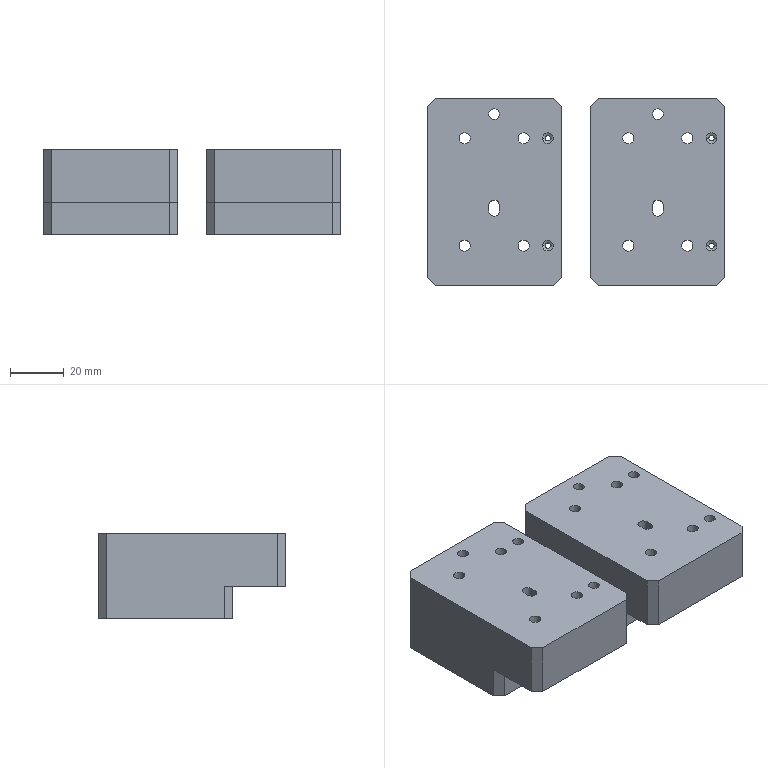NC program | NX | posted with a generic post | part box 111 x 70 x 32 mm
Lines 4642 to 5357 of 5357:
(ZLEVEL_PROFILE_1 , TOOL : D10JING)
N9276 T14 M6
N9278 G54
N9280 G17 G0 G90 X117.809 Y68.622 S9500 M3
N9282 G43 Z30. H14
N9284 Z-14.5
N9286 G94 G1 Z-16. F1000.
N9288 X116.5 Y67.866
N9290 G3 X116. Y67. R1.
N9292 G1 Y3. F1500.
N9294 G2 X114.536 Y-0.536 R5.
N9296 G1 X111.536 Y-3.536
N9298 G2 X108. Y-5. R5.
N9300 G1 X64.
N9302 G2 X60.464 Y-3.536 R5.
N9304 G1 X57.464 Y-0.536
N9306 G2 X56. Y3. R5.
N9308 G1 Y67.
N9310 G2 X57.464 Y70.536 R5.
N9312 G1 X60.464 Y73.536
N9314 G2 X64. Y75. R5.
N9316 G1 X108.
N9318 G2 X111.536 Y73.536 R5.
N9320 G1 X114.536 Y70.536
N9322 G2 X116. Y67. R5.
N9324 G3 X116.5 Y66.134 R1.
N9326 G1 X118. Y65.268
N9328 Z-14.5
N9330 G0 Z53.
N9332 X-6.809 Y1.378
N9334 Z-14.5
N9336 G1 Z-16. F1000.
N9338 X-5.5 Y2.134
N9340 G3 X-5. Y3. R1.
N9342 G1 Y67. F1500.
N9344 G2 X-3.536 Y70.536 R5.
N9346 G1 X-0.536 Y73.536
N9348 G2 X3. Y75. R5.
N9350 G1 X47.
N9352 G2 X50.536 Y73.536 R5.
N9354 G1 X53.536 Y70.536
N9356 G2 X55. Y67. R5.
N9358 G1 Y3.
N9360 G2 X53.536 Y-0.536 R5.
N9362 G1 X50.536 Y-3.536
N9364 G2 X47. Y-5. R5.
N9366 G1 X3.
N9368 G2 X-0.536 Y-3.536 R5.
N9370 G1 X-3.536 Y-0.536
N9372 G2 X-5. Y3. R5.
N9374 G1 Y67. Z-19.873
N9376 X-4.992 Y67.28 Z-19.89
N9378 X-4.969 Y67.56 Z-19.907
N9380 X-4.929 Y67.838 Z-19.924
N9382 X-4.875 Y68.113 Z-19.941
N9384 X-4.805 Y68.384 Z-19.958
N9386 X-4.719 Y68.651 Z-19.975
N9388 X-4.619 Y68.913 Z-19.992
N9390 X-4.505 Y69.169 Z-20.009
N9392 X-4.376 Y69.419 Z-20.026
N9394 X-4.234 Y69.66 Z-20.043
N9396 X-4.078 Y69.893 Z-20.06
N9398 X-3.909 Y70.117 Z-20.077
N9400 X-3.728 Y70.332 Z-20.094
N9402 X-3.536 Y70.536 Z-20.111
N9404 X-0.536 Y73.536 Z-20.368
N9406 X-0.332 Y73.728 Z-20.385
N9408 X-0.117 Y73.909 Z-20.402
N9410 X0.107 Y74.078 Z-20.419
N9412 X0.34 Y74.234 Z-20.436
N9414 X0.581 Y74.376 Z-20.453
N9416 X0.831 Y74.505 Z-20.469
N9418 X1.087 Y74.619 Z-20.486
N9420 X1.349 Y74.719 Z-20.503
N9422 X1.616 Y74.805 Z-20.52
N9424 X1.887 Y74.875 Z-20.537
N9426 X2.162 Y74.929 Z-20.554
N9428 X2.44 Y74.969 Z-20.571
N9430 X2.72 Y74.992 Z-20.588
N9432 X3. Y75. Z-20.605
N9434 X47. Z-23.268
N9436 X47.28 Y74.992 Z-23.285
N9438 X47.56 Y74.969 Z-23.302
N9440 X47.838 Y74.929 Z-23.319
N9442 X48.113 Y74.875 Z-23.336
N9444 X48.384 Y74.805 Z-23.353
N9446 X48.651 Y74.719 Z-23.37
N9448 X48.913 Y74.619 Z-23.387
N9450 X49.169 Y74.505 Z-23.404
N9452 X49.419 Y74.376 Z-23.421
N9454 X49.66 Y74.234 Z-23.438
N9456 X49.893 Y74.078 Z-23.455
N9458 X50.117 Y73.909 Z-23.472
N9460 X50.332 Y73.728 Z-23.489
N9462 X50.536 Y73.536 Z-23.506
N9464 X53.536 Y70.536 Z-23.762
N9466 X53.728 Y70.332 Z-23.779
N9468 X53.909 Y70.117 Z-23.796
N9470 X54.078 Y69.893 Z-23.813
N9472 X54.234 Y69.66 Z-23.83
N9474 X54.376 Y69.419 Z-23.847
N9476 X54.505 Y69.169 Z-23.864
N9478 X54.619 Y68.913 Z-23.881
N9480 X54.719 Y68.651 Z-23.898
N9482 X54.805 Y68.384 Z-23.915
N9484 X54.875 Y68.113 Z-23.932
N9486 X54.929 Y67.838 Z-23.949
N9488 X54.969 Y67.56 Z-23.966
N9490 X54.992 Y67.28 Z-23.983
N9492 X55. Y67. Z-24.
N9494 Y3. Z-27.873
N9496 X54.992 Y2.72 Z-27.89
N9498 X54.969 Y2.44 Z-27.907
N9500 X54.929 Y2.162 Z-27.924
N9502 X54.875 Y1.887 Z-27.941
N9504 X54.805 Y1.616 Z-27.958
N9506 X54.719 Y1.349 Z-27.975
N9508 X54.619 Y1.087 Z-27.992
N9510 X54.505 Y0.831 Z-28.009
N9512 X54.376 Y0.581 Z-28.026
N9514 X54.234 Y0.34 Z-28.043
N9516 X54.078 Y0.107 Z-28.06
N9518 X53.909 Y-0.117 Z-28.077
N9520 X53.728 Y-0.332 Z-28.094
N9522 X53.536 Y-0.536 Z-28.111
N9524 X50.536 Y-3.536 Z-28.368
N9526 X50.332 Y-3.728 Z-28.385
N9528 X50.117 Y-3.909 Z-28.402
N9530 X49.893 Y-4.078 Z-28.419
N9532 X49.66 Y-4.234 Z-28.436
N9534 X49.419 Y-4.376 Z-28.453
N9536 X49.169 Y-4.505 Z-28.469
N9538 X48.913 Y-4.619 Z-28.486
N9540 X48.651 Y-4.719 Z-28.503
N9542 X48.384 Y-4.805 Z-28.52
N9544 X48.113 Y-4.875 Z-28.537
N9546 X47.838 Y-4.929 Z-28.554
N9548 X47.56 Y-4.969 Z-28.571
N9550 X47.28 Y-4.992 Z-28.588
N9552 X47. Y-5. Z-28.605
N9554 X3. Z-31.268
N9556 X2.72 Y-4.992 Z-31.285
N9558 X2.44 Y-4.969 Z-31.302
N9560 X2.162 Y-4.929 Z-31.319
N9562 X1.887 Y-4.875 Z-31.336
N9564 X1.616 Y-4.805 Z-31.353
N9566 X1.349 Y-4.719 Z-31.37
N9568 X1.087 Y-4.619 Z-31.387
N9570 X0.831 Y-4.505 Z-31.404
N9572 X0.581 Y-4.376 Z-31.421
N9574 X0.34 Y-4.234 Z-31.438
N9576 X0.107 Y-4.078 Z-31.455
N9578 X-0.117 Y-3.909 Z-31.472
N9580 X-0.332 Y-3.728 Z-31.489
N9582 X-0.536 Y-3.536 Z-31.506
N9584 X-3.536 Y-0.536 Z-31.762
N9586 X-3.728 Y-0.332 Z-31.779
N9588 X-3.909 Y-0.117 Z-31.796
N9590 X-4.078 Y0.107 Z-31.813
N9592 X-4.234 Y0.34 Z-31.83
N9594 X-4.376 Y0.581 Z-31.847
N9596 X-4.505 Y0.831 Z-31.864
N9598 X-4.619 Y1.087 Z-31.881
N9600 X-4.719 Y1.349 Z-31.898
N9602 X-4.805 Y1.616 Z-31.915
N9604 X-4.875 Y1.887 Z-31.932
N9606 X-4.929 Y2.162 Z-31.949
N9608 X-4.969 Y2.44 Z-31.966
N9610 X-4.992 Y2.72 Z-31.983
N9612 X-5. Y3. Z-32.
N9614 Y67.
N9616 G2 X-3.536 Y70.536 R5.
N9618 G1 X-0.536 Y73.536
N9620 G2 X3. Y75. R5.
N9622 G1 X47.
N9624 G2 X50.536 Y73.536 R5.
N9626 G1 X53.536 Y70.536
N9628 G2 X55. Y67. R5.
N9630 G1 Y3.
N9632 G2 X53.536 Y-0.536 R5.
N9634 G1 X50.536 Y-3.536
N9636 G2 X47. Y-5. R5.
N9638 G1 X3.
N9640 G2 X-0.536 Y-3.536 R5.
N9642 G1 X-3.536 Y-0.536
N9644 G2 X-5. Y3. R5.
N9646 G3 X-5.5 Y3.866 R1.
N9648 G1 X-7. Y4.732
N9650 Z-30.5
N9652 G0 Z53.
N9654 X117.809 Y68.622
N9656 Z-30.5
N9658 G1 Z-32. F1000.
N9660 X116.5 Y67.866
N9662 G3 X116. Y67. R1.
N9664 G1 Y3. F1500.
N9666 G2 X114.536 Y-0.536 R5.
N9668 G1 X111.536 Y-3.536
N9670 G2 X108. Y-5. R5.
N9672 G1 X64.
N9674 G2 X60.464 Y-3.536 R5.
N9676 G1 X57.464 Y-0.536
N9678 G2 X56. Y3. R5.
N9680 G1 Y67.
N9682 G2 X57.464 Y70.536 R5.
N9684 G1 X60.464 Y73.536
N9686 G2 X64. Y75. R5.
N9688 G1 X108.
N9690 G2 X111.536 Y73.536 R5.
N9692 G1 X114.536 Y70.536
N9694 G2 X116. Y67. R5.
N9696 G3 X116.5 Y66.134 R1.
N9698 G1 X118. Y65.268
N9700 Z-30.5
N9702 G0 Z30.
N9704 M5
(DRILLING , TOOL : D6A45)
N9706 T01 M6
N9708 G54
N9710 G17 G0 G90 X106. Y55. S9500 M3
N9712 G43 Z30. H1
N9714 G94 G81 G98 Z-1.8 F250. R3.
N9716 X97.
N9718 X86. Y64.
N9720 X75. Y55.
N9722 X45.
N9724 X36.
N9726 X25. Y64.
N9728 X14. Y55.
N9730 X25. Y28.
N9732 X14. Y15.
N9734 X36.
N9736 X45.
N9738 X75.
N9740 X86. Y28.
N9742 X97. Y15.
N9744 X106.
N9746 G80
N9748 G0 X106. Y15. Z30.
N9750 M5
(DRILLING_COPY_COPY , TOOL : 4.2ZT)
N9752 T04 M6
N9754 G54
N9756 G17 G0 G90 X14. Y15. S2000 M3
N9758 G43 Z30. H4
N9760 G94 G83 G98 Z-22.762 F150. Q2. R3.
N9762 X36.
N9764 X75.
N9766 X97.
N9768 Y55. Z-34.762
N9770 X75.
N9772 X36.
N9774 X14.
N9776 G80
N9778 G0 X14. Y55. Z30.
N9780 M5
(DRILLING_COPY_COPY_1 , TOOL : 3.4ZT)
N9782 T18 M6
N9784 G54
N9786 G17 G0 G90 X25. Y64. S2000 M3
N9788 G43 Z30. H18
N9790 G94 G83 G98 Z-34.521 F150. Q2. R3.
N9792 Y28.
N9794 X45. Y15. Z-8.202
N9796 Y55.
N9798 X86. Y28. Z-34.521
N9800 Y64.
N9802 X106. Y55. Z-8.202
N9804 Y15.
N9806 G80
N9808 G0 X106. Y15. Z30.
N9810 M5
(DRILLING_COPY_COPY_1_COPY , TOOL : 2.0ZT)
N9812 T17 M6
N9814 G54
N9816 G17 G0 G90 X45. Y15. S2000 M3
N9818 G43 Z30. H17
N9820 G94 G83 G98 Z-22.101 F80. Q2. R3.
N9822 Y55. Z-34.101
N9824 X106. Y15. Z-22.101
N9826 Y55. Z-34.101
N9828 G80
N9830 G0 X106. Y55. Z30.
N9832 M5
(HOLE_MILLING , TOOL : D3)
N9834 T03 M6
N9836 G54
N9838 G17 G0 G90 X45. Y55. S9500 M3
N9840 G43 Z30. H3
N9842 Z0.5
N9844 G94 G3 X45.2 Y54.8 R0.2 F1250.
N9846 X45.4 Y55. R0.2
N9848 X45.4 Y55. Z0.3 I-0.4 J0.
N9850 X45.4 Y55. Z0.1 I-0.4 J0.
N9852 X45.4 Y55. Z-0.1 I-0.4 J0.
N9854 X45.4 Y55. Z-0.3 I-0.4 J0.
N9856 X45.4 Y55. Z-0.5 I-0.4 J0.
N9858 X45.4 Y55. Z-0.7 I-0.4 J0.
N9860 X45.4 Y55. Z-0.9 I-0.4 J0.
N9862 X45.4 Y55. Z-1.1 I-0.4 J0.
N9864 X45.4 Y55. Z-1.3 I-0.4 J0.
N9866 X45.4 Y55. Z-1.5 I-0.4 J0.
N9868 X45.4 Y55. Z-1.7 I-0.4 J0.
N9870 X45.4 Y55. Z-1.9 I-0.4 J0.
N9872 X45.4 Y55. Z-2.1 I-0.4 J0.
N9874 X45.4 Y55. Z-2.3 I-0.4 J0.
N9876 X45.4 Y55. Z-2.5 I-0.4 J0.
N9878 X45.4 Y55. Z-2.7 I-0.4 J0.
N9880 X45.4 Y55. Z-2.9 I-0.4 J0.
N9882 X45.4 Y55. Z-3.1 I-0.4 J0.
N9884 X45.4 Y55. Z-3.3 I-0.4 J0.
N9886 X45.4 Y55. Z-3.5 I-0.4 J0.
N9888 X45.4 Y55. Z-3.7 I-0.4 J0.
N9890 X45.4 Y55. Z-3.9 I-0.4 J0.
N9892 X45.4 Y55. Z-4.1 I-0.4 J0.
N9894 X45.4 Y55. Z-4.3 I-0.4 J0.
N9896 X45.4 Y55. Z-4.5 I-0.4 J0.
N9898 X45.4 Y55. Z-4.7 I-0.4 J0.
N9900 X45.4 Y55. Z-4.9 I-0.4 J0.
N9902 X45.4 Y55. Z-5.1 I-0.4 J0.
N9904 X45.4 Y55. Z-5.3 I-0.4 J0.
N9906 X45.4 Y55. Z-5.5 I-0.4 J0.
N9908 X45.4 Y55. Z-5.7 I-0.4 J0.
N9910 X45.4 Y55. Z-5.9 I-0.4 J0.
N9912 X45.4 Y55. Z-6.1 I-0.4 J0.
N9914 X45.4 Y55. Z-6.3 I-0.4 J0.
N9916 X45.4 Y55. Z-6.5 I-0.4 J0.
N9918 X45.4 Y55. Z-6.7 I-0.4 J0.
N9920 X45.4 Y55. Z-6.9 I-0.4 J0.
N9922 X44.6 Y55. Z-7. I-0.4 J0.
N9924 X45. Y54.6 R0.4
N9926 X44.6 Y55. R-0.4
N9928 X44.8 Y54.8 R0.2
N9930 X45. Y55. R0.2
N9932 G0 Z30.
N9934 Y15.
N9936 Z0.5
N9938 G3 X45.2 Y14.8 R0.2
N9940 X45.4 Y15. R0.2
N9942 X45.4 Y15. Z0.3 I-0.4 J0.
N9944 X45.4 Y15. Z0.1 I-0.4 J0.
N9946 X45.4 Y15. Z-0.1 I-0.4 J0.
N9948 X45.4 Y15. Z-0.3 I-0.4 J0.
N9950 X45.4 Y15. Z-0.5 I-0.4 J0.
N9952 X45.4 Y15. Z-0.7 I-0.4 J0.
N9954 X45.4 Y15. Z-0.9 I-0.4 J0.
N9956 X45.4 Y15. Z-1.1 I-0.4 J0.
N9958 X45.4 Y15. Z-1.3 I-0.4 J0.
N9960 X45.4 Y15. Z-1.5 I-0.4 J0.
N9962 X45.4 Y15. Z-1.7 I-0.4 J0.
N9964 X45.4 Y15. Z-1.9 I-0.4 J0.
N9966 X45.4 Y15. Z-2.1 I-0.4 J0.
N9968 X45.4 Y15. Z-2.3 I-0.4 J0.
N9970 X45.4 Y15. Z-2.5 I-0.4 J0.
N9972 X45.4 Y15. Z-2.7 I-0.4 J0.
N9974 X45.4 Y15. Z-2.9 I-0.4 J0.
N9976 X45.4 Y15. Z-3.1 I-0.4 J0.
N9978 X45.4 Y15. Z-3.3 I-0.4 J0.
N9980 X45.4 Y15. Z-3.5 I-0.4 J0.
N9982 X45.4 Y15. Z-3.7 I-0.4 J0.
N9984 X45.4 Y15. Z-3.9 I-0.4 J0.
N9986 X45.4 Y15. Z-4.1 I-0.4 J0.
N9988 X45.4 Y15. Z-4.3 I-0.4 J0.
N9990 X45.4 Y15. Z-4.5 I-0.4 J0.
N9992 X45.4 Y15. Z-4.7 I-0.4 J0.
N9994 X45.4 Y15. Z-4.9 I-0.4 J0.
N9996 X45.4 Y15. Z-5.1 I-0.4 J0.
N9998 X45.4 Y15. Z-5.3 I-0.4 J0.
N10000 X45.4 Y15. Z-5.5 I-0.4 J0.
N10002 X45.4 Y15. Z-5.7 I-0.4 J0.
N10004 X45.4 Y15. Z-5.9 I-0.4 J0.
N10006 X45.4 Y15. Z-6.1 I-0.4 J0.
N10008 X45.4 Y15. Z-6.3 I-0.4 J0.
N10010 X45.4 Y15. Z-6.5 I-0.4 J0.
N10012 X45.4 Y15. Z-6.7 I-0.4 J0.
N10014 X45.4 Y15. Z-6.9 I-0.4 J0.
N10016 X44.6 Y15. Z-7. I-0.4 J0.
N10018 X45. Y14.6 R0.4
N10020 X44.6 Y15. R-0.4
N10022 X44.8 Y14.8 R0.2
N10024 X45. Y15. R0.2
N10026 G0 Z30.
N10028 X106.
N10030 Z0.5
N10032 G3 X106.2 Y14.8 R0.2
N10034 X106.4 Y15. R0.2
N10036 X106.4 Y15. Z0.3 I-0.4 J0.
N10038 X106.4 Y15. Z0.1 I-0.4 J0.
N10040 X106.4 Y15. Z-0.1 I-0.4 J0.
N10042 X106.4 Y15. Z-0.3 I-0.4 J0.
N10044 X106.4 Y15. Z-0.5 I-0.4 J0.
N10046 X106.4 Y15. Z-0.7 I-0.4 J0.
N10048 X106.4 Y15. Z-0.9 I-0.4 J0.
N10050 X106.4 Y15. Z-1.1 I-0.4 J0.
N10052 X106.4 Y15. Z-1.3 I-0.4 J0.
N10054 X106.4 Y15. Z-1.5 I-0.4 J0.
N10056 X106.4 Y15. Z-1.7 I-0.4 J0.
N10058 X106.4 Y15. Z-1.9 I-0.4 J0.
N10060 X106.4 Y15. Z-2.1 I-0.4 J0.
N10062 X106.4 Y15. Z-2.3 I-0.4 J0.
N10064 X106.4 Y15. Z-2.5 I-0.4 J0.
N10066 X106.4 Y15. Z-2.7 I-0.4 J0.
N10068 X106.4 Y15. Z-2.9 I-0.4 J0.
N10070 X106.4 Y15. Z-3.1 I-0.4 J0.
N10072 X106.4 Y15. Z-3.3 I-0.4 J0.
N10074 X106.4 Y15. Z-3.5 I-0.4 J0.
N10076 X106.4 Y15. Z-3.7 I-0.4 J0.
N10078 X106.4 Y15. Z-3.9 I-0.4 J0.
N10080 X106.4 Y15. Z-4.1 I-0.4 J0.
N10082 X106.4 Y15. Z-4.3 I-0.4 J0.
N10084 X106.4 Y15. Z-4.5 I-0.4 J0.
N10086 X106.4 Y15. Z-4.7 I-0.4 J0.
N10088 X106.4 Y15. Z-4.9 I-0.4 J0.
N10090 X106.4 Y15. Z-5.1 I-0.4 J0.
N10092 X106.4 Y15. Z-5.3 I-0.4 J0.
N10094 X106.4 Y15. Z-5.5 I-0.4 J0.
N10096 X106.4 Y15. Z-5.7 I-0.4 J0.
N10098 X106.4 Y15. Z-5.9 I-0.4 J0.
N10100 X106.4 Y15. Z-6.1 I-0.4 J0.
N10102 X106.4 Y15. Z-6.3 I-0.4 J0.
N10104 X106.4 Y15. Z-6.5 I-0.4 J0.
N10106 X106.4 Y15. Z-6.7 I-0.4 J0.
N10108 X106.4 Y15. Z-6.9 I-0.4 J0.
N10110 X105.6 Y15. Z-7. I-0.4 J0.
N10112 X106. Y14.6 R0.4
N10114 X105.6 Y15. R-0.4
N10116 X105.8 Y14.8 R0.2
N10118 X106. Y15. R0.2
N10120 G0 Z30.
N10122 Y55.
N10124 Z0.5
N10126 G3 X106.2 Y54.8 R0.2
N10128 X106.4 Y55. R0.2
N10130 X106.4 Y55. Z0.3 I-0.4 J0.
N10132 X106.4 Y55. Z0.1 I-0.4 J0.
N10134 X106.4 Y55. Z-0.1 I-0.4 J0.
N10136 X106.4 Y55. Z-0.3 I-0.4 J0.
N10138 X106.4 Y55. Z-0.5 I-0.4 J0.
N10140 X106.4 Y55. Z-0.7 I-0.4 J0.
N10142 X106.4 Y55. Z-0.9 I-0.4 J0.
N10144 X106.4 Y55. Z-1.1 I-0.4 J0.
N10146 X106.4 Y55. Z-1.3 I-0.4 J0.
N10148 X106.4 Y55. Z-1.5 I-0.4 J0.
N10150 X106.4 Y55. Z-1.7 I-0.4 J0.
N10152 X106.4 Y55. Z-1.9 I-0.4 J0.
N10154 X106.4 Y55. Z-2.1 I-0.4 J0.
N10156 X106.4 Y55. Z-2.3 I-0.4 J0.
N10158 X106.4 Y55. Z-2.5 I-0.4 J0.
N10160 X106.4 Y55. Z-2.7 I-0.4 J0.
N10162 X106.4 Y55. Z-2.9 I-0.4 J0.
N10164 X106.4 Y55. Z-3.1 I-0.4 J0.
N10166 X106.4 Y55. Z-3.3 I-0.4 J0.
N10168 X106.4 Y55. Z-3.5 I-0.4 J0.
N10170 X106.4 Y55. Z-3.7 I-0.4 J0.
N10172 X106.4 Y55. Z-3.9 I-0.4 J0.
N10174 X106.4 Y55. Z-4.1 I-0.4 J0.
N10176 X106.4 Y55. Z-4.3 I-0.4 J0.
N10178 X106.4 Y55. Z-4.5 I-0.4 J0.
N10180 X106.4 Y55. Z-4.7 I-0.4 J0.
N10182 X106.4 Y55. Z-4.9 I-0.4 J0.
N10184 X106.4 Y55. Z-5.1 I-0.4 J0.
N10186 X106.4 Y55. Z-5.3 I-0.4 J0.
N10188 X106.4 Y55. Z-5.5 I-0.4 J0.
N10190 X106.4 Y55. Z-5.7 I-0.4 J0.
N10192 X106.4 Y55. Z-5.9 I-0.4 J0.
N10194 X106.4 Y55. Z-6.1 I-0.4 J0.
N10196 X106.4 Y55. Z-6.3 I-0.4 J0.
N10198 X106.4 Y55. Z-6.5 I-0.4 J0.
N10200 X106.4 Y55. Z-6.7 I-0.4 J0.
N10202 X106.4 Y55. Z-6.9 I-0.4 J0.
N10204 X105.6 Y55. Z-7. I-0.4 J0.
N10206 X106. Y54.6 R0.4
N10208 X105.6 Y55. R-0.4
N10210 X105.8 Y54.8 R0.2
N10212 X106. Y55. R0.2
N10214 G0 Z30.
N10216 M5
(PLANAR_MILL_COPY , TOOL : D6A45)
N10218 T01 M6
N10220 G54
N10222 G17 G0 G90 X44.134 Y14.4 S9500 M3
N10224 G43 Z30. H1
N10226 Z0.5
N10228 G94 G1 Z-1. F1250.
N10230 G3 X45. Y13.9 R1.
N10232 X46.1 Y15. R1.1
N10234 X45. Y13.9 R-1.1
N10236 X45.866 Y14.4 R1.
N10238 G1 Z0.5
N10240 G0 Z30.
N10242 X35.134 Y14.3
N10244 Z0.5
N10246 G1 Z-1.
N10248 G3 X36. Y13.8 R1.
N10250 X37.2 Y15. R1.2
N10252 X36. Y13.8 R-1.2
N10254 X36.866 Y14.3 R1.
N10256 G1 Z0.5
N10258 G0 Z30.
N10260 X13.3 Y15.866
N10262 Z0.5
N10264 G1 Z-1.
N10266 G3 X12.8 Y15. R1.
N10268 X14. Y13.8 R1.2
N10270 X12.8 Y15. R-1.2
N10272 X13.3 Y14.134 R1.
N10274 G1 Z0.5
N10276 G0 Z30.
N10278 X-1.4 Y34.134
N10280 Z0.5
N10282 G1 Z-1.
N10284 G3 X-0.9 Y35. R1.
N10286 G1 Y67.
N10288 G2 X-0.636 Y67.636 R0.9
N10290 G1 X2.364 Y70.636
N10292 G2 X3. Y70.9 R0.9
N10294 G1 X47.
N10296 G2 X47.636 Y70.636 R0.9
N10298 G1 X50.636 Y67.636
N10300 G2 X50.9 Y67. R0.9
N10302 G1 Y3.
N10304 G2 X50.636 Y2.364 R0.9
N10306 G1 X47.636 Y-0.636
N10308 G2 X47. Y-0.9 R0.9
N10310 G1 X3.
N10312 G2 X2.364 Y-0.636 R0.9
N10314 G1 X-0.636 Y2.364
N10316 G2 X-0.9 Y3. R0.9
N10318 G1 Y35.
N10320 G3 X-1.4 Y35.866 R1.
N10322 G1 Z0.5
N10324 G0 Z30.
N10326 X13.3 Y55.866
N10328 Z0.5
N10330 G1 Z-1.
N10332 G3 X12.8 Y55. R1.
N10334 X14. Y53.8 R1.2
N10336 X12.8 Y55. R-1.2
N10338 X13.3 Y54.134 R1.
N10340 G1 Z0.5
N10342 G0 Z30.
N10344 X36.866 Y55.7
N10346 Z0.5
N10348 G1 Z-1.
N10350 G3 X36. Y56.2 R1.
N10352 X34.8 Y55. R1.2
N10354 X36. Y56.2 R-1.2
N10356 X35.134 Y55.7 R1.
N10358 G1 Z0.5
N10360 G0 Z30.
N10362 X45.866 Y55.6
N10364 Z0.5
N10366 G1 Z-1.
N10368 G3 X45. Y56.1 R1.
N10370 X43.9 Y55. R1.1
N10372 X45. Y56.1 R-1.1
N10374 X44.134 Y55.6 R1.
N10376 G1 Z0.5
N10378 G0 Z30.
N10380 X75.866 Y55.7
N10382 Z0.5
N10384 G1 Z-1.
N10386 G3 X75. Y56.2 R1.
N10388 X73.8 Y55. R1.2
N10390 X75. Y56.2 R-1.2
N10392 X74.134 Y55.7 R1.
N10394 G1 Z0.5
N10396 G0 Z30.
N10398 X97.7 Y54.134
N10400 Z0.5
N10402 G1 Z-1.
N10404 G3 X98.2 Y55. R1.
N10406 X97. Y56.2 R1.2
N10408 X98.2 Y55. R-1.2
N10410 X97.7 Y55.866 R1.
N10412 G1 Z0.5
N10414 G0 Z30.
N10416 X106.6 Y54.134
N10418 Z0.5
N10420 G1 Z-1.
N10422 G3 X107.1 Y55. R1.
N10424 X106. Y56.1 R1.1
N10426 X107.1 Y55. R-1.1
N10428 X106.6 Y55.866 R1.
N10430 G1 Z0.5
N10432 G0 Z30.
N10434 X112.4 Y35.866
N10436 Z0.5
N10438 G1 Z-1.
N10440 G3 X111.9 Y35. R1.
N10442 G1 Y3.
N10444 G2 X111.636 Y2.364 R0.9
N10446 G1 X108.636 Y-0.636
N10448 G2 X108. Y-0.9 R0.9
N10450 G1 X64.
N10452 G2 X63.364 Y-0.636 R0.9
N10454 G1 X60.364 Y2.364
N10456 G2 X60.1 Y3. R0.9
N10458 G1 Y67.
N10460 G2 X60.364 Y67.636 R0.9
N10462 G1 X63.364 Y70.636
N10464 G2 X64. Y70.9 R0.9
N10466 G1 X108.
N10468 G2 X108.636 Y70.636 R0.9
N10470 G1 X111.636 Y67.636
N10472 G2 X111.9 Y67. R0.9
N10474 G1 Y35.
N10476 G3 X112.4 Y34.134 R1.
N10478 G1 Z0.5
N10480 G0 Z30.
N10482 X74.134 Y14.3
N10484 Z0.5
N10486 G1 Z-1.
N10488 G3 X75. Y13.8 R1.
N10490 X76.2 Y15. R1.2
N10492 X75. Y13.8 R-1.2
N10494 X75.866 Y14.3 R1.
N10496 G1 Z0.5
N10498 G0 Z30.
N10500 X97.7 Y14.134
N10502 Z0.5
N10504 G1 Z-1.
N10506 G3 X98.2 Y15. R1.
N10508 X97. Y16.2 R1.2
N10510 X98.2 Y15. R-1.2
N10512 X97.7 Y15.866 R1.
N10514 G1 Z0.5
N10516 G0 Z30.
N10518 X106.6 Y14.134
N10520 Z0.5
N10522 G1 Z-1.
N10524 G3 X107.1 Y15. R1.
N10526 X106. Y16.1 R1.1
N10528 X107.1 Y15. R-1.1
N10530 X106.6 Y15.866 R1.
N10532 G1 Z0.5
N10534 G0 Z30.
N10536 M5
(刀补3 , TOOL : D3)
N10538 T03 M6
N10540 G54
N10542 G17 G0 G90 X45. Y55. S9500 M3
N10544 G43 Z30. H3
N10546 Z0.5
N10548 G41 G94 G1 X45.027 Y54.904 F1250. D3
N10550 G3 X45.45 Y55. R0.222
N10552 X45.45 Y55. Z-1.5 I-0.45 J0.
N10554 X45.45 Y55. Z-3.5 I-0.45 J0.
N10556 X45.45 Y55. Z-5.5 I-0.45 J0.
N10558 X45. Y54.55 Z-7. R-0.45
N10560 X45.45 Y55. R0.45
N10562 X45. Y54.55 R-0.45
N10564 X45.096 Y54.973 R0.222
N10566 G40
N10568 G1 X45. Y55.
N10570 G0 Z30.
N10572 Y15.
N10574 Z0.5
N10576 G41 G1 X45.027 Y14.904
N10578 G3 X45.45 Y15. R0.222
N10580 X45.45 Y15. Z-1.5 I-0.45 J0.
N10582 X45.45 Y15. Z-3.5 I-0.45 J0.
N10584 X45.45 Y15. Z-5.5 I-0.45 J0.
N10586 X45. Y14.55 Z-7. R-0.45
N10588 X45.45 Y15. R0.45
N10590 X45. Y14.55 R-0.45
N10592 X45.096 Y14.973 R0.222
N10594 G40
N10596 G1 X45. Y15.
N10598 G0 Z30.
N10600 X106.
N10602 Z0.5
N10604 G41 G1 X106.027 Y14.904
N10606 G3 X106.45 Y15. R0.222
N10608 X106.45 Y15. Z-1.5 I-0.45 J0.
N10610 X106.45 Y15. Z-3.5 I-0.45 J0.
N10612 X106.45 Y15. Z-5.5 I-0.45 J0.
N10614 X106. Y14.55 Z-7. R-0.45
N10616 X106.45 Y15. R0.45
N10618 X106. Y14.55 R-0.45
N10620 X106.096 Y14.973 R0.222
N10622 G40
N10624 G1 X106. Y15.
N10626 G0 Z30.
N10628 Y55.
N10630 Z0.5
N10632 G41 G1 X106.027 Y54.904
N10634 G3 X106.45 Y55. R0.222
N10636 X106.45 Y55. Z-1.5 I-0.45 J0.
N10638 X106.45 Y55. Z-3.5 I-0.45 J0.
N10640 X106.45 Y55. Z-5.5 I-0.45 J0.
N10642 X106. Y54.55 Z-7. R-0.45
N10644 X106.45 Y55. R0.45
N10646 X106. Y54.55 R-0.45
N10648 X106.096 Y54.973 R0.222
N10650 G40
N10652 G1 X106. Y55.
N10654 G0 Z30.
N10656 M5
N10658 M2